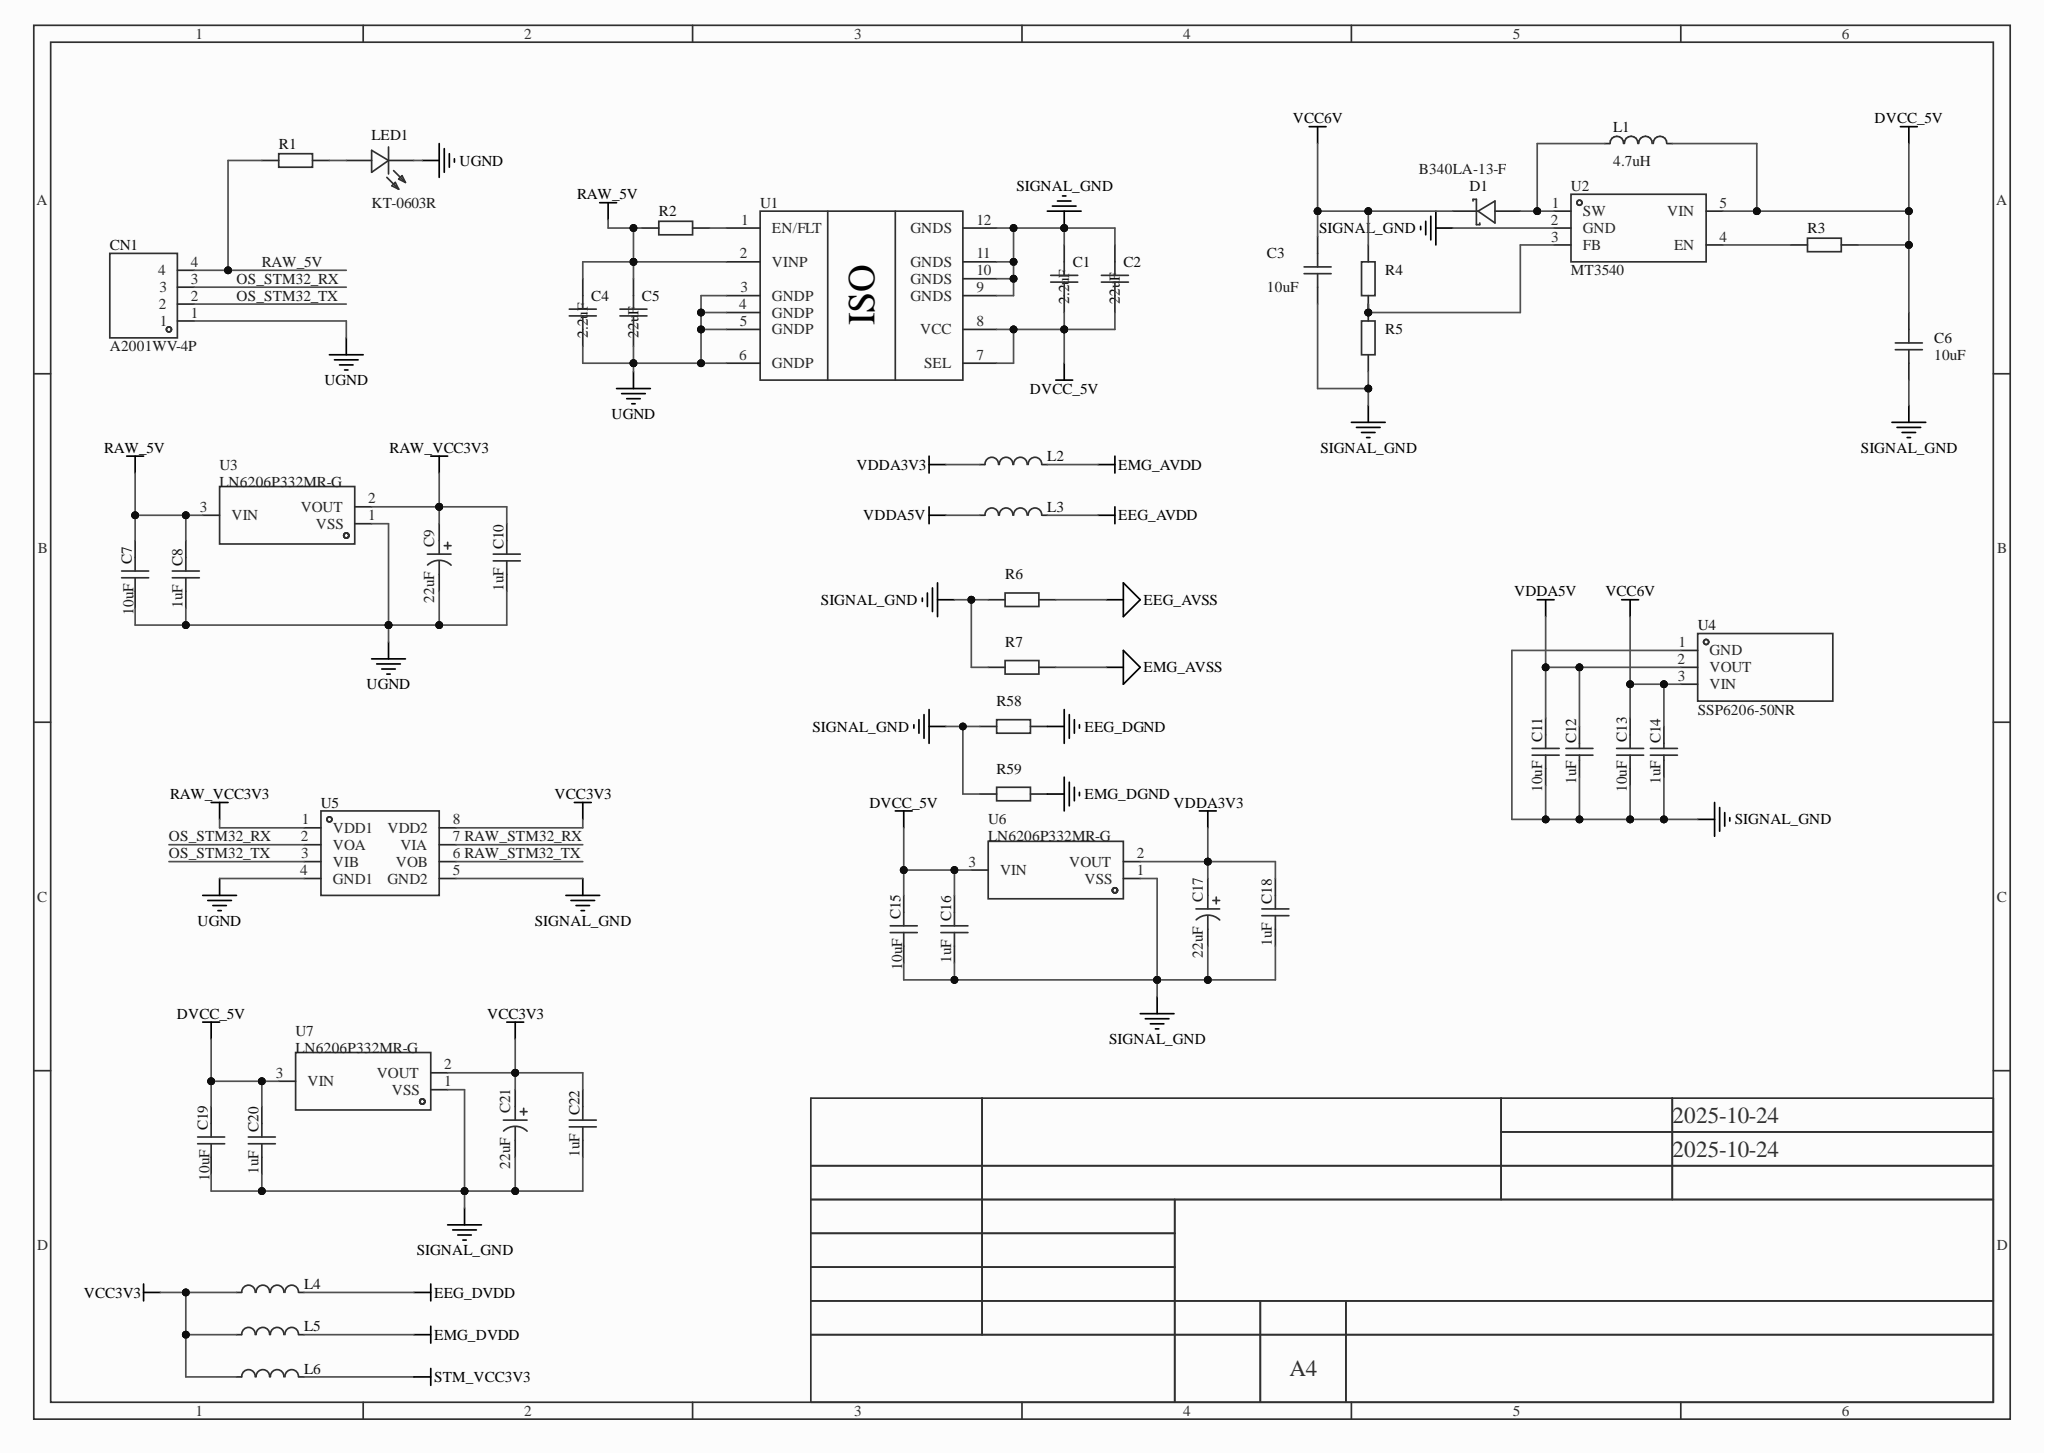Circuit board | Altium Designer | 212 parts | 123 nets | one sheet of the schematic
Parts on this sheet (reference | value | footprint):
C2 | 22uF | C0603
C3 | 10uF | C0603
C5 | 22uF | C0603
C6 | 10uF | C0603
C7 | 10uF | C0603
C8 | 1uF | C0402
C9 | 22uF | CAP-SMD_L3.2-W1.6
C10 | 1uF | C0402
C11 | 10uF | C0603
C12 | 1uF | C0402
C13 | 10uF | C0603
C14 | 1uF | C0402
C15 | 10uF | C0603
C16 | 1uF | C0402
C17 | 22uF | CAP-SMD_L3.2-W1.6
C18 | 1uF | C0402
C19 | 10uF | C0603
C20 | 1uF | C0402
C21 | 22uF | CAP-SMD_L3.2-W1.6
C22 | 1uF | C0402
CN1 | A2001WV-4P | CONN-TH_A2001WV-4P
D1 | B340LA-13-F | SMA_L4.3-W2.6-LS5.2-RD
L1 | 4.7uH | IND-SMD_L4.0-W4.0_FNR40XXS
L2 | BLM15PD121SN1D | L0402
L3 | BLM15PD121SN1D | L0402
L4 | BLM15PD121SN1D | L0402
L5 | BLM15PD121SN1D | L0402
L6 | BLM15PD121SN1D | L0402
LED1 | KT-0603R | LED0603-RD
R1 | R0603
R2 | R0603
R3 | R0402
R4 | R0402
R5 | R0402
R6 | R0402
R7 | R0402
R58 | R0402
R59 | R0402
U1 | VSON-FCRLF
U2 | MT3540 | SOT-23-5_L3.0-W1.7-P0.95-LS2.8-BR
U3 | LN6206P332MR-G | SOT-23-3_L2.9-W1.3-P1.90-LS2.4-BR
U4 | SSP6206-50NR | SOT-23-3_L2.9-W1.3-P1.90-LS2.4-BR
U5 | SOIC-8_L4.9-W3.9-P1.27-LS6.0-BL
U6 | LN6206P332MR-G | SOT-23-3_L2.9-W1.3-P1.90-LS2.4-BR
U7 | LN6206P332MR-G | SOT-23-3_L2.9-W1.3-P1.90-LS2.4-BR
Nets of these parts (net: part-pin ...):
VDDA5V: C11-2 C12-2 L3-1 U4-2
VDDA3V3: C17-1 C18-2 L2-1 U6-2
VCC6V: C3-2 C13-2 C14-2 D1-1 R4-2 U4-3
VCC3V3: C21-1 C22-2 L4-1 L5-1 L6-1 U5-8 U7-2
UGND: C5-1 C7-1 C8-1 C9-2 C10-1 CN1-1 LED1-1 U1-3 U1-4 U1-5 U1-6 U3-1 U5-4
STM_VCC3V3: L6-2
SIGNAL_GND: C2-2 C3-1 C6-1 C11-1 C12-1 C13-1 C14-1 C15-1 C16-1 C17-2 C18-1 C19-1 C20-1 C21-2 C22-1 R5-1 R6-2 R7-2 R58-2 R59-2 U1-9 U1-10 U1-11 U1-12 U2-2 U4-1 U5-5 U6-1 U7-1
RAW_VCC3V3: C9-1 C10-2 U3-2 U5-1
RAW_STM32_TX: U5-6
RAW_STM32_RX: U5-7
RAW_5V: C5-2 C7-2 C8-2 CN1-4 R1-1 R2-1 U1-2 U3-3
OS_STM32_TX: CN1-2 U5-3
OS_STM32_RX: CN1-3 U5-2
NetR4_1: R4-1 R5-2 U2-3
NetR3_1: R3-1 U2-4
NetR2_2: R2-2 U1-1
NetLED1_2: LED1-2 R1-2
NetD1_2: D1-2 L1-1 U2-1
EMG_DVDD: L5-2
EMG_DGND: R59-1
EMG_AVSS1: R7-1
EMG_AVDD1: L2-2
EEG_DVDD_1: L4-2
EEG_DGND_1: R58-1
EEG_AVSS1: R6-1
EEG_AVDD1: L3-2
DVCC_5V: C2-1 C6-2 C15-2 C16-2 C19-2 C20-2 L1-2 R3-2 U1-7 U1-8 U2-5 U6-3 U7-3